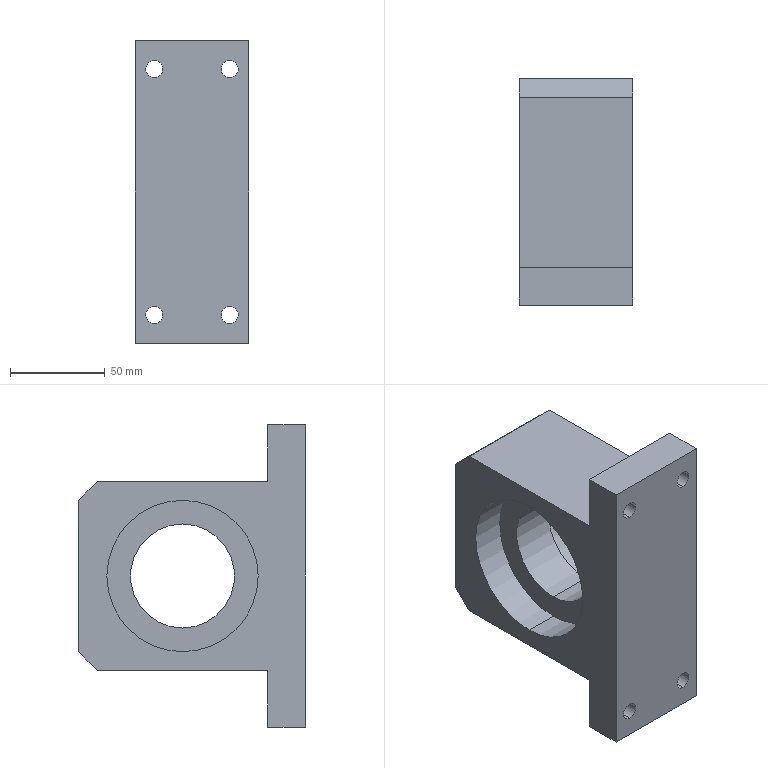Part | SolidWorks | features BaseBody 1 | 1 solid | 28 faces | box 60 x 120 x 160 mm | volume 542935 mm3 | cylinder 14 | plane 14 | commonest cylinder face diameters 9 x8 80 x4 55 x2
STEP:
#1=CARTESIAN_POINT('',(-12.,5.,40.));
#2=VERTEX_POINT('',#1);
#3=CARTESIAN_POINT('',(-12.,5.,-40.));
#4=VERTEX_POINT('',#3);
#5=CARTESIAN_POINT('',(-12.,5.,0.));
#6=DIRECTION('',(1.,0.,0.));
#7=DIRECTION('',(0.,0.,-1.));
#8=AXIS2_PLACEMENT_3D('',#5,#6,#7);
#9=CIRCLE('',#8,40.);
#10=EDGE_CURVE('',#2,#4,#9,.T.);
#11=ORIENTED_EDGE('',*,*,#10,.T.);
#12=CARTESIAN_POINT('',(-30.,5.,-40.));
#13=VERTEX_POINT('',#12);
#14=CARTESIAN_POINT('',(-12.,5.,-40.));
#15=DIRECTION('',(-1.,0.,0.));
#16=VECTOR('',#15,1000.);
#17=LINE('',#14,#16);
#18=EDGE_CURVE('',#4,#13,#17,.T.);
#19=ORIENTED_EDGE('',*,*,#18,.T.);
#20=CARTESIAN_POINT('',(-30.,5.,40.));
#21=VERTEX_POINT('',#20);
#22=CARTESIAN_POINT('',(-30.,5.,0.));
#23=DIRECTION('',(1.,0.,0.));
#24=DIRECTION('',(0.,0.,-1.));
#25=AXIS2_PLACEMENT_3D('',#22,#23,#24);
#26=CIRCLE('',#25,40.);
#27=EDGE_CURVE('',#21,#13,#26,.T.);
#28=ORIENTED_EDGE('',*,*,#27,.F.);
#29=CARTESIAN_POINT('',(-12.,5.,40.));
#30=DIRECTION('',(-1.,0.,0.));
#31=VECTOR('',#30,1000.);
#32=LINE('',#29,#31);
#33=EDGE_CURVE('',#2,#21,#32,.T.);
#34=ORIENTED_EDGE('',*,*,#33,.F.);
#35=EDGE_LOOP('',(#11,#19,#28,#34));
#36=FACE_OUTER_BOUND('',#35,.T.);
#37=CARTESIAN_POINT('',(-12.,5.,0.));
#38=DIRECTION('',(-1.,0.,0.));
#39=DIRECTION('',(0.,0.,1.));
#40=AXIS2_PLACEMENT_3D('',#37,#38,#39);
#41=CYLINDRICAL_SURFACE('',#40,40.);
#42=ADVANCED_FACE('',(#36),#41,.F.);
#43=CARTESIAN_POINT('',(12.,5.,40.));
#44=VERTEX_POINT('',#43);
#45=CARTESIAN_POINT('',(12.,5.,-40.));
#46=VERTEX_POINT('',#45);
#47=CARTESIAN_POINT('',(12.,5.,0.));
#48=DIRECTION('',(1.,0.,0.));
#49=DIRECTION('',(0.,0.,-1.));
#50=AXIS2_PLACEMENT_3D('',#47,#48,#49);
#51=CIRCLE('',#50,40.);
#52=EDGE_CURVE('',#44,#46,#51,.T.);
#53=ORIENTED_EDGE('',*,*,#52,.F.);
#54=CARTESIAN_POINT('',(30.,5.,40.));
#55=VERTEX_POINT('',#54);
#56=CARTESIAN_POINT('',(12.,5.,40.));
#57=DIRECTION('',(1.,0.,0.));
#58=VECTOR('',#57,1000.);
#59=LINE('',#56,#58);
#60=EDGE_CURVE('',#44,#55,#59,.T.);
#61=ORIENTED_EDGE('',*,*,#60,.T.);
#62=CARTESIAN_POINT('',(30.,5.,-40.));
#63=VERTEX_POINT('',#62);
#64=CARTESIAN_POINT('',(30.,5.,0.));
#65=DIRECTION('',(1.,0.,0.));
#66=DIRECTION('',(0.,0.,-1.));
#67=AXIS2_PLACEMENT_3D('',#64,#65,#66);
#68=CIRCLE('',#67,40.);
#69=EDGE_CURVE('',#55,#63,#68,.T.);
#70=ORIENTED_EDGE('',*,*,#69,.T.);
#71=CARTESIAN_POINT('',(12.,5.,-40.));
#72=DIRECTION('',(1.,0.,0.));
#73=VECTOR('',#72,1000.);
#74=LINE('',#71,#73);
#75=EDGE_CURVE('',#46,#63,#74,.T.);
#76=ORIENTED_EDGE('',*,*,#75,.F.);
#77=EDGE_LOOP('',(#53,#61,#70,#76));
#78=FACE_OUTER_BOUND('',#77,.T.);
#79=CARTESIAN_POINT('',(12.,5.,0.));
#80=DIRECTION('',(1.,0.,0.));
#81=DIRECTION('',(0.,0.,-1.));
#82=AXIS2_PLACEMENT_3D('',#79,#80,#81);
#83=CYLINDRICAL_SURFACE('',#82,40.);
#84=ADVANCED_FACE('',(#78),#83,.F.);
#85=CARTESIAN_POINT('',(20.,-60.,-69.5));
#86=VERTEX_POINT('',#85);
#87=CARTESIAN_POINT('',(20.,-60.,-60.5));
#88=VERTEX_POINT('',#87);
#89=CARTESIAN_POINT('',(20.,-60.,-65.));
#90=DIRECTION('',(0.,1.,0.));
#91=DIRECTION('',(0.,0.,1.));
#92=AXIS2_PLACEMENT_3D('',#89,#90,#91);
#93=CIRCLE('',#92,4.5);
#94=EDGE_CURVE('',#86,#88,#93,.T.);
#95=ORIENTED_EDGE('',*,*,#94,.F.);
#96=CARTESIAN_POINT('',(20.,-40.,-69.5));
#97=VERTEX_POINT('',#96);
#98=CARTESIAN_POINT('',(20.,-100.,-69.5));
#99=DIRECTION('',(0.,1.,0.));
#100=VECTOR('',#99,1000.);
#101=LINE('',#98,#100);
#102=EDGE_CURVE('',#86,#97,#101,.T.);
#103=ORIENTED_EDGE('',*,*,#102,.T.);
#104=CARTESIAN_POINT('',(20.,-40.,-60.5));
#105=VERTEX_POINT('',#104);
#106=CARTESIAN_POINT('',(20.,-40.,-65.));
#107=DIRECTION('',(0.,-1.,0.));
#108=DIRECTION('',(0.,0.,-1.));
#109=AXIS2_PLACEMENT_3D('',#106,#107,#108);
#110=CIRCLE('',#109,4.5);
#111=EDGE_CURVE('',#105,#97,#110,.T.);
#112=ORIENTED_EDGE('',*,*,#111,.F.);
#113=CARTESIAN_POINT('',(20.,-100.,-60.5));
#114=DIRECTION('',(0.,1.,0.));
#115=VECTOR('',#114,1000.);
#116=LINE('',#113,#115);
#117=EDGE_CURVE('',#88,#105,#116,.T.);
#118=ORIENTED_EDGE('',*,*,#117,.F.);
#119=EDGE_LOOP('',(#95,#103,#112,#118));
#120=FACE_OUTER_BOUND('',#119,.T.);
#121=CARTESIAN_POINT('',(20.,-100.,-65.));
#122=DIRECTION('',(0.,1.,0.));
#123=DIRECTION('',(0.,0.,1.));
#124=AXIS2_PLACEMENT_3D('',#121,#122,#123);
#125=CYLINDRICAL_SURFACE('',#124,4.5);
#126=ADVANCED_FACE('',(#120),#125,.F.);
#127=CARTESIAN_POINT('',(-20.,-60.,-69.5));
#128=VERTEX_POINT('',#127);
#129=CARTESIAN_POINT('',(-20.,-60.,-60.5));
#130=VERTEX_POINT('',#129);
#131=CARTESIAN_POINT('',(-20.,-60.,-65.));
#132=DIRECTION('',(0.,1.,0.));
#133=DIRECTION('',(0.,0.,1.));
#134=AXIS2_PLACEMENT_3D('',#131,#132,#133);
#135=CIRCLE('',#134,4.5);
#136=EDGE_CURVE('',#128,#130,#135,.T.);
#137=ORIENTED_EDGE('',*,*,#136,.F.);
#138=CARTESIAN_POINT('',(-20.,-40.,-69.5));
#139=VERTEX_POINT('',#138);
#140=CARTESIAN_POINT('',(-20.,-100.,-69.5));
#141=DIRECTION('',(0.,1.,0.));
#142=VECTOR('',#141,1000.);
#143=LINE('',#140,#142);
#144=EDGE_CURVE('',#128,#139,#143,.T.);
#145=ORIENTED_EDGE('',*,*,#144,.T.);
#146=CARTESIAN_POINT('',(-20.,-40.,-60.5));
#147=VERTEX_POINT('',#146);
#148=CARTESIAN_POINT('',(-20.,-40.,-65.));
#149=DIRECTION('',(0.,-1.,0.));
#150=DIRECTION('',(0.,0.,-1.));
#151=AXIS2_PLACEMENT_3D('',#148,#149,#150);
#152=CIRCLE('',#151,4.5);
#153=EDGE_CURVE('',#147,#139,#152,.T.);
#154=ORIENTED_EDGE('',*,*,#153,.F.);
#155=CARTESIAN_POINT('',(-20.,-100.,-60.5));
#156=DIRECTION('',(0.,1.,0.));
#157=VECTOR('',#156,1000.);
#158=LINE('',#155,#157);
#159=EDGE_CURVE('',#130,#147,#158,.T.);
#160=ORIENTED_EDGE('',*,*,#159,.F.);
#161=EDGE_LOOP('',(#137,#145,#154,#160));
#162=FACE_OUTER_BOUND('',#161,.T.);
#163=CARTESIAN_POINT('',(-20.,-100.,-65.));
#164=DIRECTION('',(0.,1.,0.));
#165=DIRECTION('',(0.,0.,1.));
#166=AXIS2_PLACEMENT_3D('',#163,#164,#165);
#167=CYLINDRICAL_SURFACE('',#166,4.5);
#168=ADVANCED_FACE('',(#162),#167,.F.);
#169=CARTESIAN_POINT('',(-20.,-60.,60.5));
#170=VERTEX_POINT('',#169);
#171=CARTESIAN_POINT('',(-20.,-60.,69.5));
#172=VERTEX_POINT('',#171);
#173=CARTESIAN_POINT('',(-20.,-60.,65.));
#174=DIRECTION('',(0.,1.,0.));
#175=DIRECTION('',(0.,0.,1.));
#176=AXIS2_PLACEMENT_3D('',#173,#174,#175);
#177=CIRCLE('',#176,4.5);
#178=EDGE_CURVE('',#170,#172,#177,.T.);
#179=ORIENTED_EDGE('',*,*,#178,.F.);
#180=CARTESIAN_POINT('',(-20.,-40.,60.5));
#181=VERTEX_POINT('',#180);
#182=CARTESIAN_POINT('',(-20.,-100.,60.5));
#183=DIRECTION('',(0.,1.,0.));
#184=VECTOR('',#183,1000.);
#185=LINE('',#182,#184);
#186=EDGE_CURVE('',#170,#181,#185,.T.);
#187=ORIENTED_EDGE('',*,*,#186,.T.);
#188=CARTESIAN_POINT('',(-20.,-40.,69.5));
#189=VERTEX_POINT('',#188);
#190=CARTESIAN_POINT('',(-20.,-40.,65.));
#191=DIRECTION('',(0.,-1.,0.));
#192=DIRECTION('',(0.,0.,-1.));
#193=AXIS2_PLACEMENT_3D('',#190,#191,#192);
#194=CIRCLE('',#193,4.5);
#195=EDGE_CURVE('',#189,#181,#194,.T.);
#196=ORIENTED_EDGE('',*,*,#195,.F.);
#197=CARTESIAN_POINT('',(-20.,-100.,69.5));
#198=DIRECTION('',(0.,1.,0.));
#199=VECTOR('',#198,1000.);
#200=LINE('',#197,#199);
#201=EDGE_CURVE('',#172,#189,#200,.T.);
#202=ORIENTED_EDGE('',*,*,#201,.F.);
#203=EDGE_LOOP('',(#179,#187,#196,#202));
#204=FACE_OUTER_BOUND('',#203,.T.);
#205=CARTESIAN_POINT('',(-20.,-100.,65.));
#206=DIRECTION('',(0.,1.,0.));
#207=DIRECTION('',(0.,0.,1.));
#208=AXIS2_PLACEMENT_3D('',#205,#206,#207);
#209=CYLINDRICAL_SURFACE('',#208,4.5);
#210=ADVANCED_FACE('',(#204),#209,.F.);
#211=CARTESIAN_POINT('',(20.,-60.,60.5));
#212=VERTEX_POINT('',#211);
#213=CARTESIAN_POINT('',(20.,-60.,69.5));
#214=VERTEX_POINT('',#213);
#215=CARTESIAN_POINT('',(20.,-60.,65.));
#216=DIRECTION('',(0.,1.,0.));
#217=DIRECTION('',(0.,0.,1.));
#218=AXIS2_PLACEMENT_3D('',#215,#216,#217);
#219=CIRCLE('',#218,4.5);
#220=EDGE_CURVE('',#212,#214,#219,.T.);
#221=ORIENTED_EDGE('',*,*,#220,.F.);
#222=CARTESIAN_POINT('',(20.,-40.,60.5));
#223=VERTEX_POINT('',#222);
#224=CARTESIAN_POINT('',(20.,-100.,60.5));
#225=DIRECTION('',(0.,1.,0.));
#226=VECTOR('',#225,1000.);
#227=LINE('',#224,#226);
#228=EDGE_CURVE('',#212,#223,#227,.T.);
#229=ORIENTED_EDGE('',*,*,#228,.T.);
#230=CARTESIAN_POINT('',(20.,-40.,69.5));
#231=VERTEX_POINT('',#230);
#232=CARTESIAN_POINT('',(20.,-40.,65.));
#233=DIRECTION('',(0.,-1.,0.));
#234=DIRECTION('',(0.,0.,-1.));
#235=AXIS2_PLACEMENT_3D('',#232,#233,#234);
#236=CIRCLE('',#235,4.5);
#237=EDGE_CURVE('',#231,#223,#236,.T.);
#238=ORIENTED_EDGE('',*,*,#237,.F.);
#239=CARTESIAN_POINT('',(20.,-100.,69.5));
#240=DIRECTION('',(0.,1.,0.));
#241=VECTOR('',#240,1000.);
#242=LINE('',#239,#241);
#243=EDGE_CURVE('',#214,#231,#242,.T.);
#244=ORIENTED_EDGE('',*,*,#243,.F.);
#245=EDGE_LOOP('',(#221,#229,#238,#244));
#246=FACE_OUTER_BOUND('',#245,.T.);
#247=CARTESIAN_POINT('',(20.,-100.,65.));
#248=DIRECTION('',(0.,1.,0.));
#249=DIRECTION('',(0.,0.,1.));
#250=AXIS2_PLACEMENT_3D('',#247,#248,#249);
#251=CYLINDRICAL_SURFACE('',#250,4.5);
#252=ADVANCED_FACE('',(#246),#251,.F.);
#253=CARTESIAN_POINT('',(-12.,5.,27.5));
#254=VERTEX_POINT('',#253);
#255=CARTESIAN_POINT('',(-12.,5.,-27.5));
#256=VERTEX_POINT('',#255);
#257=CARTESIAN_POINT('',(-12.,5.,0.));
#258=DIRECTION('',(1.,0.,0.));
#259=DIRECTION('',(0.,0.,1.));
#260=AXIS2_PLACEMENT_3D('',#257,#258,#259);
#261=CIRCLE('',#260,27.5);
#262=EDGE_CURVE('',#254,#256,#261,.T.);
#263=ORIENTED_EDGE('',*,*,#262,.F.);
#264=CARTESIAN_POINT('',(12.,5.,27.5));
#265=VERTEX_POINT('',#264);
#266=CARTESIAN_POINT('',(-30.,5.,27.5));
#267=DIRECTION('',(1.,0.,0.));
#268=VECTOR('',#267,1000.);
#269=LINE('',#266,#268);
#270=EDGE_CURVE('',#254,#265,#269,.T.);
#271=ORIENTED_EDGE('',*,*,#270,.T.);
#272=CARTESIAN_POINT('',(12.,5.,-27.5));
#273=VERTEX_POINT('',#272);
#274=CARTESIAN_POINT('',(12.,5.,0.));
#275=DIRECTION('',(-1.,0.,0.));
#276=DIRECTION('',(0.,0.,-1.));
#277=AXIS2_PLACEMENT_3D('',#274,#275,#276);
#278=CIRCLE('',#277,27.5);
#279=EDGE_CURVE('',#273,#265,#278,.T.);
#280=ORIENTED_EDGE('',*,*,#279,.F.);
#281=CARTESIAN_POINT('',(-30.,5.,-27.5));
#282=DIRECTION('',(1.,0.,0.));
#283=VECTOR('',#282,1000.);
#284=LINE('',#281,#283);
#285=EDGE_CURVE('',#256,#273,#284,.T.);
#286=ORIENTED_EDGE('',*,*,#285,.F.);
#287=EDGE_LOOP('',(#263,#271,#280,#286));
#288=FACE_OUTER_BOUND('',#287,.T.);
#289=CARTESIAN_POINT('',(-30.,5.,0.));
#290=DIRECTION('',(1.,0.,0.));
#291=DIRECTION('',(0.,0.,-1.));
#292=AXIS2_PLACEMENT_3D('',#289,#290,#291);
#293=CYLINDRICAL_SURFACE('',#292,27.5);
#294=ADVANCED_FACE('',(#288),#293,.F.);
#295=ORIENTED_EDGE('',*,*,#270,.F.);
#296=CARTESIAN_POINT('',(-12.,5.,0.));
#297=DIRECTION('',(1.,0.,0.));
#298=DIRECTION('',(0.,0.,1.));
#299=AXIS2_PLACEMENT_3D('',#296,#297,#298);
#300=CIRCLE('',#299,27.5);
#301=EDGE_CURVE('',#256,#254,#300,.T.);
#302=ORIENTED_EDGE('',*,*,#301,.F.);
#303=ORIENTED_EDGE('',*,*,#285,.T.);
#304=CARTESIAN_POINT('',(12.,5.,0.));
#305=DIRECTION('',(-1.,0.,0.));
#306=DIRECTION('',(0.,0.,-1.));
#307=AXIS2_PLACEMENT_3D('',#304,#305,#306);
#308=CIRCLE('',#307,27.5);
#309=EDGE_CURVE('',#265,#273,#308,.T.);
#310=ORIENTED_EDGE('',*,*,#309,.F.);
#311=EDGE_LOOP('',(#295,#302,#303,#310));
#312=FACE_OUTER_BOUND('',#311,.T.);
#313=CARTESIAN_POINT('',(-30.,5.,0.));
#314=DIRECTION('',(1.,0.,0.));
#315=DIRECTION('',(0.,0.,-1.));
#316=AXIS2_PLACEMENT_3D('',#313,#314,#315);
#317=CYLINDRICAL_SURFACE('',#316,27.5);
#318=ADVANCED_FACE('',(#312),#317,.F.);
#319=CARTESIAN_POINT('',(30.,5.,0.));
#320=DIRECTION('',(1.,0.,0.));
#321=DIRECTION('',(0.,0.,-1.));
#322=AXIS2_PLACEMENT_3D('',#319,#320,#321);
#323=CIRCLE('',#322,40.);
#324=EDGE_CURVE('',#63,#55,#323,.T.);
#325=ORIENTED_EDGE('',*,*,#324,.F.);
#326=ORIENTED_EDGE('',*,*,#69,.F.);
#327=EDGE_LOOP('',(#325,#326));
#328=FACE_BOUND('',#327,.T.);
#329=CARTESIAN_POINT('',(30.,-40.,-50.));
#330=VERTEX_POINT('',#329);
#331=CARTESIAN_POINT('',(30.,50.,-50.));
#332=VERTEX_POINT('',#331);
#333=CARTESIAN_POINT('',(30.,60.,-50.));
#334=DIRECTION('',(0.,1.,0.));
#335=VECTOR('',#334,1000.);
#336=LINE('',#333,#335);
#337=EDGE_CURVE('',#330,#332,#336,.T.);
#338=ORIENTED_EDGE('',*,*,#337,.T.);
#339=CARTESIAN_POINT('',(30.,60.,-40.));
#340=VERTEX_POINT('',#339);
#341=CARTESIAN_POINT('',(30.,50.,-50.));
#342=DIRECTION('',(0.,0.7071,0.7071));
#343=VECTOR('',#342,1000.);
#344=LINE('',#341,#343);
#345=EDGE_CURVE('',#332,#340,#344,.T.);
#346=ORIENTED_EDGE('',*,*,#345,.T.);
#347=CARTESIAN_POINT('',(30.,60.,40.));
#348=VERTEX_POINT('',#347);
#349=CARTESIAN_POINT('',(30.,60.,-80.));
#350=DIRECTION('',(0.,0.,-1.));
#351=VECTOR('',#350,1000.);
#352=LINE('',#349,#351);
#353=EDGE_CURVE('',#348,#340,#352,.T.);
#354=ORIENTED_EDGE('',*,*,#353,.F.);
#355=CARTESIAN_POINT('',(30.,50.,50.));
#356=VERTEX_POINT('',#355);
#357=CARTESIAN_POINT('',(30.,50.,50.));
#358=DIRECTION('',(0.,-0.7071,0.7071));
#359=VECTOR('',#358,1000.);
#360=LINE('',#357,#359);
#361=EDGE_CURVE('',#348,#356,#360,.T.);
#362=ORIENTED_EDGE('',*,*,#361,.T.);
#363=CARTESIAN_POINT('',(30.,-40.,50.));
#364=VERTEX_POINT('',#363);
#365=CARTESIAN_POINT('',(30.,60.,50.));
#366=DIRECTION('',(0.,-1.,0.));
#367=VECTOR('',#366,1000.);
#368=LINE('',#365,#367);
#369=EDGE_CURVE('',#356,#364,#368,.T.);
#370=ORIENTED_EDGE('',*,*,#369,.T.);
#371=CARTESIAN_POINT('',(30.,-40.,80.));
#372=VERTEX_POINT('',#371);
#373=CARTESIAN_POINT('',(30.,-40.,-80.));
#374=DIRECTION('',(0.,0.,1.));
#375=VECTOR('',#374,1000.);
#376=LINE('',#373,#375);
#377=EDGE_CURVE('',#364,#372,#376,.T.);
#378=ORIENTED_EDGE('',*,*,#377,.T.);
#379=CARTESIAN_POINT('',(30.,-60.,80.));
#380=VERTEX_POINT('',#379);
#381=CARTESIAN_POINT('',(30.,60.,80.));
#382=DIRECTION('',(0.,-1.,0.));
#383=VECTOR('',#382,1000.);
#384=LINE('',#381,#383);
#385=EDGE_CURVE('',#372,#380,#384,.T.);
#386=ORIENTED_EDGE('',*,*,#385,.T.);
#387=CARTESIAN_POINT('',(30.,-60.,-80.));
#388=VERTEX_POINT('',#387);
#389=CARTESIAN_POINT('',(30.,-60.,-80.));
#390=DIRECTION('',(0.,0.,-1.));
#391=VECTOR('',#390,1000.);
#392=LINE('',#389,#391);
#393=EDGE_CURVE('',#380,#388,#392,.T.);
#394=ORIENTED_EDGE('',*,*,#393,.T.);
#395=CARTESIAN_POINT('',(30.,-40.,-80.));
#396=VERTEX_POINT('',#395);
#397=CARTESIAN_POINT('',(30.,60.,-80.));
#398=DIRECTION('',(0.,-1.,0.));
#399=VECTOR('',#398,1000.);
#400=LINE('',#397,#399);
#401=EDGE_CURVE('',#396,#388,#400,.T.);
#402=ORIENTED_EDGE('',*,*,#401,.F.);
#403=CARTESIAN_POINT('',(30.,-40.,-80.));
#404=DIRECTION('',(0.,0.,1.));
#405=VECTOR('',#404,1000.);
#406=LINE('',#403,#405);
#407=EDGE_CURVE('',#396,#330,#406,.T.);
#408=ORIENTED_EDGE('',*,*,#407,.T.);
#409=EDGE_LOOP('',(#338,#346,#354,#362,#370,#378,#386,#394,#402,#408));
#410=FACE_OUTER_BOUND('',#409,.T.);
#411=CARTESIAN_POINT('',(30.,60.,-80.));
#412=DIRECTION('',(-1.,0.,0.));
#413=DIRECTION('',(0.,0.,1.));
#414=AXIS2_PLACEMENT_3D('',#411,#412,#413);
#415=PLANE('',#414);
#416=ADVANCED_FACE('',(#328,#410),#415,.F.);
#417=CARTESIAN_POINT('',(-30.,-40.,-80.));
#418=VERTEX_POINT('',#417);
#419=CARTESIAN_POINT('',(-30.,-60.,-80.));
#420=VERTEX_POINT('',#419);
#421=CARTESIAN_POINT('',(-30.,60.,-80.));
#422=DIRECTION('',(0.,-1.,0.));
#423=VECTOR('',#422,1000.);
#424=LINE('',#421,#423);
#425=EDGE_CURVE('',#418,#420,#424,.T.);
#426=ORIENTED_EDGE('',*,*,#425,.F.);
#427=CARTESIAN_POINT('',(-60.,-40.,-80.));
#428=DIRECTION('',(1.,0.,0.));
#429=VECTOR('',#428,1000.);
#430=LINE('',#427,#429);
#431=EDGE_CURVE('',#418,#396,#430,.T.);
#432=ORIENTED_EDGE('',*,*,#431,.T.);
#433=ORIENTED_EDGE('',*,*,#401,.T.);
#434=CARTESIAN_POINT('',(-30.,-60.,-80.));
#435=DIRECTION('',(-1.,0.,0.));
#436=VECTOR('',#435,1000.);
#437=LINE('',#434,#436);
#438=EDGE_CURVE('',#388,#420,#437,.T.);
#439=ORIENTED_EDGE('',*,*,#438,.T.);
#440=EDGE_LOOP('',(#426,#432,#433,#439));
#441=FACE_OUTER_BOUND('',#440,.T.);
#442=CARTESIAN_POINT('',(-30.,60.,-80.));
#443=DIRECTION('',(0.,0.,1.));
#444=DIRECTION('',(1.,0.,0.));
#445=AXIS2_PLACEMENT_3D('',#442,#443,#444);
#446=PLANE('',#445);
#447=ADVANCED_FACE('',(#441),#446,.F.);
#448=ORIENTED_EDGE('',*,*,#27,.T.);
#449=CARTESIAN_POINT('',(-30.,5.,0.));
#450=DIRECTION('',(1.,0.,0.));
#451=DIRECTION('',(0.,0.,-1.));
#452=AXIS2_PLACEMENT_3D('',#449,#450,#451);
#453=CIRCLE('',#452,40.);
#454=EDGE_CURVE('',#13,#21,#453,.T.);
#455=ORIENTED_EDGE('',*,*,#454,.T.);
#456=EDGE_LOOP('',(#448,#455));
#457=FACE_BOUND('',#456,.T.);
#458=CARTESIAN_POINT('',(-30.,60.,-40.));
#459=VERTEX_POINT('',#458);
#460=CARTESIAN_POINT('',(-30.,60.,40.));
#461=VERTEX_POINT('',#460);
#462=CARTESIAN_POINT('',(-30.,60.,-80.));
#463=DIRECTION('',(0.,0.,1.));
#464=VECTOR('',#463,1000.);
#465=LINE('',#462,#464);
#466=EDGE_CURVE('',#459,#461,#465,.T.);
#467=ORIENTED_EDGE('',*,*,#466,.F.);
#468=CARTESIAN_POINT('',(-30.,50.,-50.));
#469=VERTEX_POINT('',#468);
#470=CARTESIAN_POINT('',(-30.,50.,-50.));
#471=DIRECTION('',(0.,-0.7071,-0.7071));
#472=VECTOR('',#471,1000.);
#473=LINE('',#470,#472);
#474=EDGE_CURVE('',#459,#469,#473,.T.);
#475=ORIENTED_EDGE('',*,*,#474,.T.);
#476=CARTESIAN_POINT('',(-30.,-40.,-50.));
#477=VERTEX_POINT('',#476);
#478=CARTESIAN_POINT('',(-30.,60.,-50.));
#479=DIRECTION('',(0.,-1.,0.));
#480=VECTOR('',#479,1000.);
#481=LINE('',#478,#480);
#482=EDGE_CURVE('',#469,#477,#481,.T.);
#483=ORIENTED_EDGE('',*,*,#482,.T.);
#484=CARTESIAN_POINT('',(-30.,-40.,-80.));
#485=DIRECTION('',(0.,0.,-1.));
#486=VECTOR('',#485,1000.);
#487=LINE('',#484,#486);
#488=EDGE_CURVE('',#477,#418,#487,.T.);
#489=ORIENTED_EDGE('',*,*,#488,.T.);
#490=ORIENTED_EDGE('',*,*,#425,.T.);
#491=CARTESIAN_POINT('',(-30.,-60.,80.));
#492=VERTEX_POINT('',#491);
#493=CARTESIAN_POINT('',(-30.,-60.,-80.));
#494=DIRECTION('',(0.,0.,1.));
#495=VECTOR('',#494,1000.);
#496=LINE('',#493,#495);
#497=EDGE_CURVE('',#420,#492,#496,.T.);
#498=ORIENTED_EDGE('',*,*,#497,.T.);
#499=CARTESIAN_POINT('',(-30.,-40.,80.));
#500=VERTEX_POINT('',#499);
#501=CARTESIAN_POINT('',(-30.,60.,80.));
#502=DIRECTION('',(0.,-1.,0.));
#503=VECTOR('',#502,1000.);
#504=LINE('',#501,#503);
#505=EDGE_CURVE('',#500,#492,#504,.T.);
#506=ORIENTED_EDGE('',*,*,#505,.F.);
#507=CARTESIAN_POINT('',(-30.,-40.,50.));
#508=VERTEX_POINT('',#507);
#509=CARTESIAN_POINT('',(-30.,-40.,-80.));
#510=DIRECTION('',(0.,0.,-1.));
#511=VECTOR('',#510,1000.);
#512=LINE('',#509,#511);
#513=EDGE_CURVE('',#500,#508,#512,.T.);
#514=ORIENTED_EDGE('',*,*,#513,.T.);
#515=CARTESIAN_POINT('',(-30.,50.,50.));
#516=VERTEX_POINT('',#515);
#517=CARTESIAN_POINT('',(-30.,60.,50.));
#518=DIRECTION('',(0.,1.,0.));
#519=VECTOR('',#518,1000.);
#520=LINE('',#517,#519);
#521=EDGE_CURVE('',#508,#516,#520,.T.);
#522=ORIENTED_EDGE('',*,*,#521,.T.);
#523=CARTESIAN_POINT('',(-30.,50.,50.));
#524=DIRECTION('',(0.,0.7071,-0.7071));
#525=VECTOR('',#524,1000.);
#526=LINE('',#523,#525);
#527=EDGE_CURVE('',#516,#461,#526,.T.);
#528=ORIENTED_EDGE('',*,*,#527,.T.);
#529=EDGE_LOOP('',(#467,#475,#483,#489,#490,#498,#506,#514,#522,#528));
#530=FACE_OUTER_BOUND('',#529,.T.);
#531=CARTESIAN_POINT('',(-30.,60.,-80.));
#532=DIRECTION('',(1.,0.,0.));
#533=DIRECTION('',(0.,0.,-1.));
#534=AXIS2_PLACEMENT_3D('',#531,#532,#533);
#535=PLANE('',#534);
#536=ADVANCED_FACE('',(#457,#530),#535,.F.);
#537=ORIENTED_EDGE('',*,*,#385,.F.);
#538=CARTESIAN_POINT('',(-60.,-40.,80.));
#539=DIRECTION('',(1.,0.,0.));
#540=VECTOR('',#539,1000.);
#541=LINE('',#538,#540);
#542=EDGE_CURVE('',#500,#372,#541,.T.);
#543=ORIENTED_EDGE('',*,*,#542,.F.);
#544=ORIENTED_EDGE('',*,*,#505,.T.);
#545=CARTESIAN_POINT('',(-30.,-60.,80.));
#546=DIRECTION('',(1.,0.,0.));
#547=VECTOR('',#546,1000.);
#548=LINE('',#545,#547);
#549=EDGE_CURVE('',#492,#380,#548,.T.);
#550=ORIENTED_EDGE('',*,*,#549,.T.);
#551=EDGE_LOOP('',(#537,#543,#544,#550));
#552=FACE_OUTER_BOUND('',#551,.T.);
#553=CARTESIAN_POINT('',(-30.,60.,80.));
#554=DIRECTION('',(0.,0.,-1.));
#555=DIRECTION('',(-1.,0.,0.));
#556=AXIS2_PLACEMENT_3D('',#553,#554,#555);
#557=PLANE('',#556);
#558=ADVANCED_FACE('',(#552),#557,.F.);
#559=ORIENTED_EDGE('',*,*,#353,.T.);
#560=CARTESIAN_POINT('',(-30.,60.,-40.));
#561=DIRECTION('',(-1.,0.,0.));
#562=VECTOR('',#561,1000.);
#563=LINE('',#560,#562);
#564=EDGE_CURVE('',#340,#459,#563,.T.);
#565=ORIENTED_EDGE('',*,*,#564,.T.);
#566=ORIENTED_EDGE('',*,*,#466,.T.);
#567=CARTESIAN_POINT('',(30.,60.,40.));
#568=DIRECTION('',(1.,0.,0.));
#569=VECTOR('',#568,1000.);
#570=LINE('',#567,#569);
#571=EDGE_CURVE('',#461,#348,#570,.T.);
#572=ORIENTED_EDGE('',*,*,#571,.T.);
#573=EDGE_LOOP('',(#559,#565,#566,#572));
#574=FACE_OUTER_BOUND('',#573,.T.);
#575=CARTESIAN_POINT('',(0.,60.,0.));
#576=DIRECTION('',(0.,1.,0.));
#577=DIRECTION('',(0.,0.,1.));
#578=AXIS2_PLACEMENT_3D('',#575,#576,#577);
#579=PLANE('',#578);
#580=ADVANCED_FACE('',(#574),#579,.T.);
#581=CARTESIAN_POINT('',(-20.,-60.,65.));
#582=DIRECTION('',(0.,1.,0.));
#583=DIRECTION('',(0.,0.,1.));
#584=AXIS2_PLACEMENT_3D('',#581,#582,#583);
#585=CIRCLE('',#584,4.5);
#586=EDGE_CURVE('',#172,#170,#585,.T.);
#587=ORIENTED_EDGE('',*,*,#586,.T.);
#588=ORIENTED_EDGE('',*,*,#178,.T.);
#589=EDGE_LOOP('',(#587,#588));
#590=FACE_BOUND('',#589,.T.);
#591=CARTESIAN_POINT('',(20.,-60.,65.));
#592=DIRECTION('',(0.,1.,0.));
#593=DIRECTION('',(0.,0.,1.));
#594=AXIS2_PLACEMENT_3D('',#591,#592,#593);
#595=CIRCLE('',#594,4.5);
#596=EDGE_CURVE('',#214,#212,#595,.T.);
#597=ORIENTED_EDGE('',*,*,#596,.T.);
#598=ORIENTED_EDGE('',*,*,#220,.T.);
#599=EDGE_LOOP('',(#597,#598));
#600=FACE_BOUND('',#599,.T.);
#601=CARTESIAN_POINT('',(20.,-60.,-65.));
#602=DIRECTION('',(0.,1.,0.));
#603=DIRECTION('',(0.,0.,1.));
#604=AXIS2_PLACEMENT_3D('',#601,#602,#603);
#605=CIRCLE('',#604,4.5);
#606=EDGE_CURVE('',#88,#86,#605,.T.);
#607=ORIENTED_EDGE('',*,*,#606,.T.);
#608=ORIENTED_EDGE('',*,*,#94,.T.);
#609=EDGE_LOOP('',(#607,#608));
#610=FACE_BOUND('',#609,.T.);
#611=CARTESIAN_POINT('',(-20.,-60.,-65.));
#612=DIRECTION('',(0.,1.,0.));
#613=DIRECTION('',(0.,0.,1.));
#614=AXIS2_PLACEMENT_3D('',#611,#612,#613);
#615=CIRCLE('',#614,4.5);
#616=EDGE_CURVE('',#130,#128,#615,.T.);
#617=ORIENTED_EDGE('',*,*,#616,.T.);
#618=ORIENTED_EDGE('',*,*,#136,.T.);
#619=EDGE_LOOP('',(#617,#618));
#620=FACE_BOUND('',#619,.T.);
#621=ORIENTED_EDGE('',*,*,#393,.F.);
#622=ORIENTED_EDGE('',*,*,#549,.F.);
#623=ORIENTED_EDGE('',*,*,#497,.F.);
#624=ORIENTED_EDGE('',*,*,#438,.F.);
#625=EDGE_LOOP('',(#621,#622,#623,#624));
#626=FACE_OUTER_BOUND('',#625,.T.);
#627=CARTESIAN_POINT('',(0.,-60.,0.));
#628=DIRECTION('',(0.,1.,0.));
#629=DIRECTION('',(0.,0.,1.));
#630=AXIS2_PLACEMENT_3D('',#627,#628,#629);
#631=PLANE('',#630);
#632=ADVANCED_FACE('',(#590,#600,#610,#620,#626),#631,.F.);
#633=ORIENTED_EDGE('',*,*,#111,.T.);
#634=CARTESIAN_POINT('',(20.,-40.,-65.));
#635=DIRECTION('',(0.,-1.,0.));
#636=DIRECTION('',(0.,0.,-1.));
#637=AXIS2_PLACEMENT_3D('',#634,#635,#636);
#638=CIRCLE('',#637,4.5);
#639=EDGE_CURVE('',#97,#105,#638,.T.);
#640=ORIENTED_EDGE('',*,*,#639,.T.);
#641=EDGE_LOOP('',(#633,#640));
#642=FACE_BOUND('',#641,.T.);
#643=ORIENTED_EDGE('',*,*,#153,.T.);
#644=CARTESIAN_POINT('',(-20.,-40.,-65.));
#645=DIRECTION('',(0.,-1.,0.));
#646=DIRECTION('',(0.,0.,-1.));
#647=AXIS2_PLACEMENT_3D('',#644,#645,#646);
#648=CIRCLE('',#647,4.5);
#649=EDGE_CURVE('',#139,#147,#648,.T.);
#650=ORIENTED_EDGE('',*,*,#649,.T.);
#651=EDGE_LOOP('',(#643,#650));
#652=FACE_BOUND('',#651,.T.);
#653=ORIENTED_EDGE('',*,*,#431,.F.);
#654=ORIENTED_EDGE('',*,*,#488,.F.);
#655=CARTESIAN_POINT('',(-60.,-40.,-50.));
#656=DIRECTION('',(1.,0.,0.));
#657=VECTOR('',#656,1000.);
#658=LINE('',#655,#657);
#659=EDGE_CURVE('',#477,#330,#658,.T.);
#660=ORIENTED_EDGE('',*,*,#659,.T.);
#661=ORIENTED_EDGE('',*,*,#407,.F.);
#662=EDGE_LOOP('',(#653,#654,#660,#661));
#663=FACE_OUTER_BOUND('',#662,.T.);
#664=CARTESIAN_POINT('',(-60.,-40.,-80.));
#665=DIRECTION('',(0.,-1.,0.));
#666=DIRECTION('',(0.,0.,-1.));
#667=AXIS2_PLACEMENT_3D('',#664,#665,#666);
#668=PLANE('',#667);
#669=ADVANCED_FACE('',(#642,#652,#663),#668,.F.);
#670=ORIENTED_EDGE('',*,*,#482,.F.);
#671=CARTESIAN_POINT('',(30.,50.,-50.));
#672=DIRECTION('',(1.,0.,0.));
#673=VECTOR('',#672,1000.);
#674=LINE('',#671,#673);
#675=EDGE_CURVE('',#469,#332,#674,.T.);
#676=ORIENTED_EDGE('',*,*,#675,.T.);
#677=ORIENTED_EDGE('',*,*,#337,.F.);
#678=ORIENTED_EDGE('',*,*,#659,.F.);
#679=EDGE_LOOP('',(#670,#676,#677,#678));
#680=FACE_OUTER_BOUND('',#679,.T.);
#681=CARTESIAN_POINT('',(-60.,60.,-50.));
#682=DIRECTION('',(0.,0.,1.));
#683=DIRECTION('',(0.,-1.,0.));
#684=AXIS2_PLACEMENT_3D('',#681,#682,#683);
#685=PLANE('',#684);
#686=ADVANCED_FACE('',(#680),#685,.F.);
#687=ORIENTED_EDGE('',*,*,#195,.T.);
#688=CARTESIAN_POINT('',(-20.,-40.,65.));
#689=DIRECTION('',(0.,-1.,0.));
#690=DIRECTION('',(0.,0.,-1.));
#691=AXIS2_PLACEMENT_3D('',#688,#689,#690);
#692=CIRCLE('',#691,4.5);
#693=EDGE_CURVE('',#181,#189,#692,.T.);
#694=ORIENTED_EDGE('',*,*,#693,.T.);
#695=EDGE_LOOP('',(#687,#694));
#696=FACE_BOUND('',#695,.T.);
#697=ORIENTED_EDGE('',*,*,#237,.T.);
#698=CARTESIAN_POINT('',(20.,-40.,65.));
#699=DIRECTION('',(0.,-1.,0.));
#700=DIRECTION('',(0.,0.,-1.));
#701=AXIS2_PLACEMENT_3D('',#698,#699,#700);
#702=CIRCLE('',#701,4.5);
#703=EDGE_CURVE('',#223,#231,#702,.T.);
#704=ORIENTED_EDGE('',*,*,#703,.T.);
#705=EDGE_LOOP('',(#697,#704));
#706=FACE_BOUND('',#705,.T.);
#707=CARTESIAN_POINT('',(-60.,-40.,50.));
#708=DIRECTION('',(1.,0.,0.));
#709=VECTOR('',#708,1000.);
#710=LINE('',#707,#709);
#711=EDGE_CURVE('',#508,#364,#710,.T.);
#712=ORIENTED_EDGE('',*,*,#711,.F.);
#713=ORIENTED_EDGE('',*,*,#513,.F.);
#714=ORIENTED_EDGE('',*,*,#542,.T.);
#715=ORIENTED_EDGE('',*,*,#377,.F.);
#716=EDGE_LOOP('',(#712,#713,#714,#715));
#717=FACE_OUTER_BOUND('',#716,.T.);
#718=CARTESIAN_POINT('',(-60.,-40.,80.));
#719=DIRECTION('',(0.,-1.,0.));
#720=DIRECTION('',(0.,0.,-1.));
#721=AXIS2_PLACEMENT_3D('',#718,#719,#720);
#722=PLANE('',#721);
#723=ADVANCED_FACE('',(#696,#706,#717),#722,.F.);
#724=ORIENTED_EDGE('',*,*,#369,.F.);
#725=CARTESIAN_POINT('',(-30.,50.,50.));
#726=DIRECTION('',(-1.,0.,0.));
#727=VECTOR('',#726,1000.);
#728=LINE('',#725,#727);
#729=EDGE_CURVE('',#356,#516,#728,.T.);
#730=ORIENTED_EDGE('',*,*,#729,.T.);
#731=ORIENTED_EDGE('',*,*,#521,.F.);
#732=ORIENTED_EDGE('',*,*,#711,.T.);
#733=EDGE_LOOP('',(#724,#730,#731,#732));
#734=FACE_OUTER_BOUND('',#733,.T.);
#735=CARTESIAN_POINT('',(-60.,60.,50.));
#736=DIRECTION('',(0.,0.,-1.));
#737=DIRECTION('',(0.,1.,0.));
#738=AXIS2_PLACEMENT_3D('',#735,#736,#737);
#739=PLANE('',#738);
#740=ADVANCED_FACE('',(#734),#739,.F.);
#741=ORIENTED_EDGE('',*,*,#228,.F.);
#742=ORIENTED_EDGE('',*,*,#596,.F.);
#743=ORIENTED_EDGE('',*,*,#243,.T.);
#744=ORIENTED_EDGE('',*,*,#703,.F.);
#745=EDGE_LOOP('',(#741,#742,#743,#744));
#746=FACE_OUTER_BOUND('',#745,.T.);
#747=CARTESIAN_POINT('',(20.,-100.,65.));
#748=DIRECTION('',(0.,1.,0.));
#749=DIRECTION('',(0.,0.,1.));
#750=AXIS2_PLACEMENT_3D('',#747,#748,#749);
#751=CYLINDRICAL_SURFACE('',#750,4.5);
#752=ADVANCED_FACE('',(#746),#751,.F.);
#753=ORIENTED_EDGE('',*,*,#186,.F.);
#754=ORIENTED_EDGE('',*,*,#586,.F.);
#755=ORIENTED_EDGE('',*,*,#201,.T.);
#756=ORIENTED_EDGE('',*,*,#693,.F.);
#757=EDGE_LOOP('',(#753,#754,#755,#756));
#758=FACE_OUTER_BOUND('',#757,.T.);
#759=CARTESIAN_POINT('',(-20.,-100.,65.));
#760=DIRECTION('',(0.,1.,0.));
#761=DIRECTION('',(0.,0.,1.));
#762=AXIS2_PLACEMENT_3D('',#759,#760,#761);
#763=CYLINDRICAL_SURFACE('',#762,4.5);
#764=ADVANCED_FACE('',(#758),#763,.F.);
#765=ORIENTED_EDGE('',*,*,#144,.F.);
#766=ORIENTED_EDGE('',*,*,#616,.F.);
#767=ORIENTED_EDGE('',*,*,#159,.T.);
#768=ORIENTED_EDGE('',*,*,#649,.F.);
#769=EDGE_LOOP('',(#765,#766,#767,#768));
#770=FACE_OUTER_BOUND('',#769,.T.);
#771=CARTESIAN_POINT('',(-20.,-100.,-65.));
#772=DIRECTION('',(0.,1.,0.));
#773=DIRECTION('',(0.,0.,1.));
#774=AXIS2_PLACEMENT_3D('',#771,#772,#773);
#775=CYLINDRICAL_SURFACE('',#774,4.5);
#776=ADVANCED_FACE('',(#770),#775,.F.);
#777=ORIENTED_EDGE('',*,*,#102,.F.);
#778=ORIENTED_EDGE('',*,*,#606,.F.);
#779=ORIENTED_EDGE('',*,*,#117,.T.);
#780=ORIENTED_EDGE('',*,*,#639,.F.);
#781=EDGE_LOOP('',(#777,#778,#779,#780));
#782=FACE_OUTER_BOUND('',#781,.T.);
#783=CARTESIAN_POINT('',(20.,-100.,-65.));
#784=DIRECTION('',(0.,1.,0.));
#785=DIRECTION('',(0.,0.,1.));
#786=AXIS2_PLACEMENT_3D('',#783,#784,#785);
#787=CYLINDRICAL_SURFACE('',#786,4.5);
#788=ADVANCED_FACE('',(#782),#787,.F.);
#789=ORIENTED_EDGE('',*,*,#474,.F.);
#790=ORIENTED_EDGE('',*,*,#564,.F.);
#791=ORIENTED_EDGE('',*,*,#345,.F.);
#792=ORIENTED_EDGE('',*,*,#675,.F.);
#793=EDGE_LOOP('',(#789,#790,#791,#792));
#794=FACE_OUTER_BOUND('',#793,.T.);
#795=CARTESIAN_POINT('',(-60.,50.,-50.));
#796=DIRECTION('',(0.,0.7071,-0.7071));
#797=DIRECTION('',(-1.,0.,0.));
#798=AXIS2_PLACEMENT_3D('',#795,#796,#797);
#799=PLANE('',#798);
#800=ADVANCED_FACE('',(#794),#799,.T.);
#801=ORIENTED_EDGE('',*,*,#361,.F.);
#802=ORIENTED_EDGE('',*,*,#571,.F.);
#803=ORIENTED_EDGE('',*,*,#527,.F.);
#804=ORIENTED_EDGE('',*,*,#729,.F.);
#805=EDGE_LOOP('',(#801,#802,#803,#804));
#806=FACE_OUTER_BOUND('',#805,.T.);
#807=CARTESIAN_POINT('',(-60.,50.,50.));
#808=DIRECTION('',(0.,0.7071,0.7071));
#809=DIRECTION('',(1.,0.,0.));
#810=AXIS2_PLACEMENT_3D('',#807,#808,#809);
#811=PLANE('',#810);
#812=ADVANCED_FACE('',(#806),#811,.T.);
#813=CARTESIAN_POINT('',(12.,5.,0.));
#814=DIRECTION('',(1.,0.,0.));
#815=DIRECTION('',(0.,0.,-1.));
#816=AXIS2_PLACEMENT_3D('',#813,#814,#815);
#817=CIRCLE('',#816,40.);
#818=EDGE_CURVE('',#46,#44,#817,.T.);
#819=ORIENTED_EDGE('',*,*,#818,.T.);
#820=ORIENTED_EDGE('',*,*,#52,.T.);
#821=EDGE_LOOP('',(#819,#820));
#822=FACE_OUTER_BOUND('',#821,.T.);
#823=ORIENTED_EDGE('',*,*,#279,.T.);
#824=ORIENTED_EDGE('',*,*,#309,.T.);
#825=EDGE_LOOP('',(#823,#824));
#826=FACE_BOUND('',#825,.T.);
#827=CARTESIAN_POINT('',(12.,5.,0.));
#828=DIRECTION('',(1.,0.,0.));
#829=DIRECTION('',(0.,0.,-1.));
#830=AXIS2_PLACEMENT_3D('',#827,#828,#829);
#831=PLANE('',#830);
#832=ADVANCED_FACE('',(#822,#826),#831,.T.);
#833=ORIENTED_EDGE('',*,*,#60,.F.);
#834=ORIENTED_EDGE('',*,*,#818,.F.);
#835=ORIENTED_EDGE('',*,*,#75,.T.);
#836=ORIENTED_EDGE('',*,*,#324,.T.);
#837=EDGE_LOOP('',(#833,#834,#835,#836));
#838=FACE_OUTER_BOUND('',#837,.T.);
#839=CARTESIAN_POINT('',(12.,5.,0.));
#840=DIRECTION('',(1.,0.,0.));
#841=DIRECTION('',(0.,0.,-1.));
#842=AXIS2_PLACEMENT_3D('',#839,#840,#841);
#843=CYLINDRICAL_SURFACE('',#842,40.);
#844=ADVANCED_FACE('',(#838),#843,.F.);
#845=ORIENTED_EDGE('',*,*,#10,.F.);
#846=CARTESIAN_POINT('',(-12.,5.,0.));
#847=DIRECTION('',(1.,0.,0.));
#848=DIRECTION('',(0.,0.,-1.));
#849=AXIS2_PLACEMENT_3D('',#846,#847,#848);
#850=CIRCLE('',#849,40.);
#851=EDGE_CURVE('',#4,#2,#850,.T.);
#852=ORIENTED_EDGE('',*,*,#851,.F.);
#853=EDGE_LOOP('',(#845,#852));
#854=FACE_OUTER_BOUND('',#853,.T.);
#855=ORIENTED_EDGE('',*,*,#301,.T.);
#856=ORIENTED_EDGE('',*,*,#262,.T.);
#857=EDGE_LOOP('',(#855,#856));
#858=FACE_BOUND('',#857,.T.);
#859=CARTESIAN_POINT('',(-12.,5.,0.));
#860=DIRECTION('',(-1.,0.,0.));
#861=DIRECTION('',(0.,0.,-1.));
#862=AXIS2_PLACEMENT_3D('',#859,#860,#861);
#863=PLANE('',#862);
#864=ADVANCED_FACE('',(#854,#858),#863,.T.);
#865=ORIENTED_EDGE('',*,*,#18,.F.);
#866=ORIENTED_EDGE('',*,*,#851,.T.);
#867=ORIENTED_EDGE('',*,*,#33,.T.);
#868=ORIENTED_EDGE('',*,*,#454,.F.);
#869=EDGE_LOOP('',(#865,#866,#867,#868));
#870=FACE_OUTER_BOUND('',#869,.T.);
#871=CARTESIAN_POINT('',(-12.,5.,0.));
#872=DIRECTION('',(-1.,0.,0.));
#873=DIRECTION('',(0.,0.,1.));
#874=AXIS2_PLACEMENT_3D('',#871,#872,#873);
#875=CYLINDRICAL_SURFACE('',#874,40.);
#876=ADVANCED_FACE('',(#870),#875,.F.);
#877=CLOSED_SHELL('',(#42,#84,#126,#168,#210,#252,#294,#318,#416,#447,#536,#558,#580,#632,#669,#686,#723,#740,#752,#764,#776,#788,#800,#812,#832,#844,#864,#876));
#878=MANIFOLD_SOLID_BREP('',#877);
#879=CARTESIAN_POINT('',(0.,0.,0.));
#880=DIRECTION('',(0.,0.,1.));
#881=DIRECTION('',(1.,0.,0.));
#882=AXIS2_PLACEMENT_3D('',#879,#880,#881);
#883=(LENGTH_UNIT()NAMED_UNIT(*)SI_UNIT(.MILLI.,.METRE.));
#884=UNCERTAINTY_MEASURE_WITH_UNIT(LENGTH_MEASURE(0.00001),#883,'','');
#885=(NAMED_UNIT(*)PLANE_ANGLE_UNIT()SI_UNIT($,.RADIAN.));
#886=(NAMED_UNIT(*)SI_UNIT($,.STERADIAN.)SOLID_ANGLE_UNIT());
#887=(GEOMETRIC_REPRESENTATION_CONTEXT(3)GLOBAL_UNCERTAINTY_ASSIGNED_CONTEXT((#884))GLOBAL_UNIT_ASSIGNED_CONTEXT((#883,#885,#886))REPRESENTATION_CONTEXT('',''));
#888=ADVANCED_BREP_SHAPE_REPRESENTATION('',(#878,#882),#887);